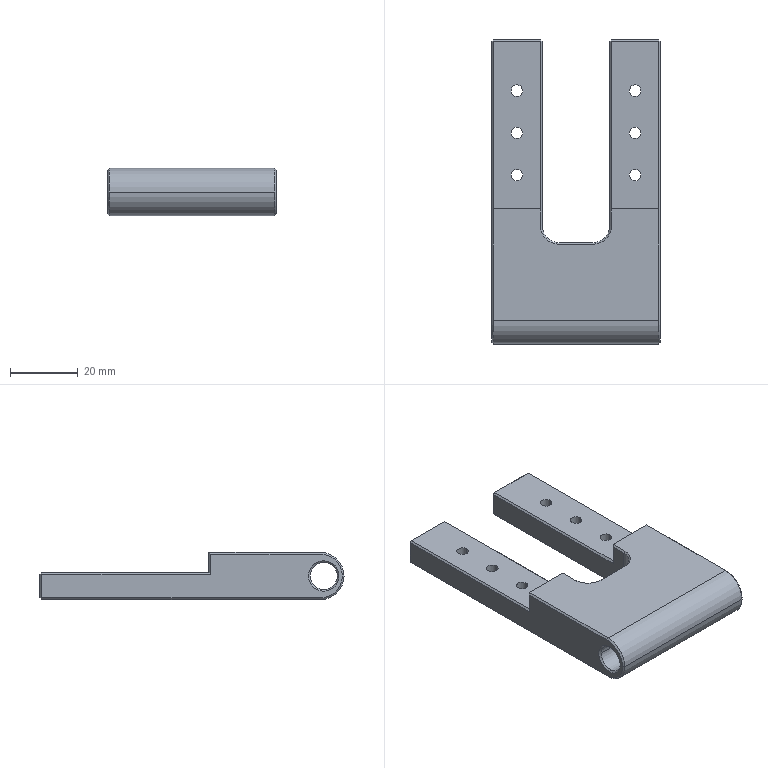Part | STEP file | BPSP-11-16 Pusher Plate_Default | 1 solid | 95 faces | box 50 x 90 x 14 mm | volume 32757 mm3 | plane 53 | cylinder 30 | cone 12 | commonest cylinder face diameters 3.4 x12 6.5 x12 8 x2 10 x2 14 x2